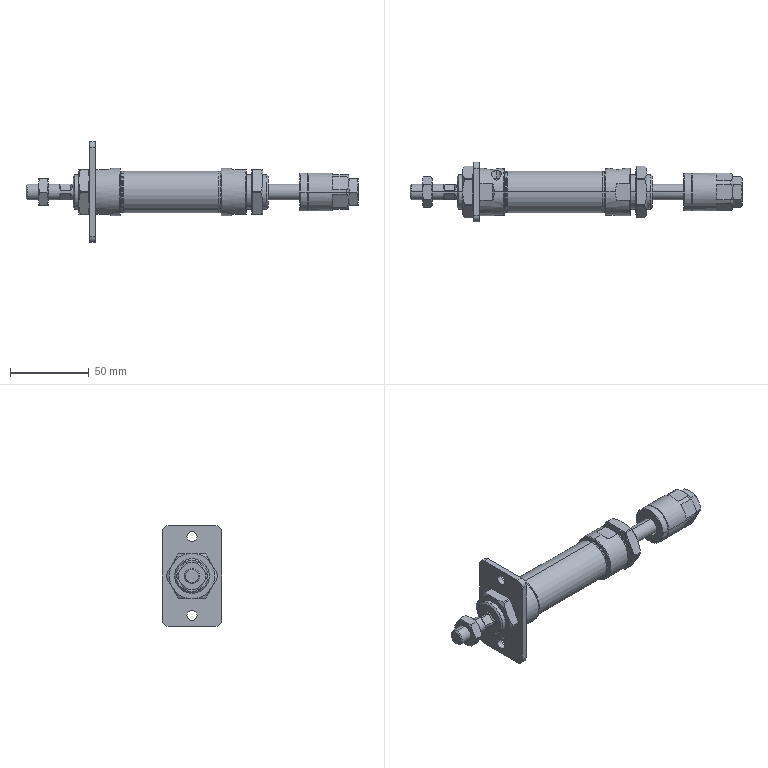Part | STEP file | 8 solids | 272 faces | box 211 x 38 x 64 mm | volume 90003 mm3 | plane 102 | cone 82 | cylinder 74 | torus 14 | commonest cylinder face diameters 33 x12 6.5 x10 10 x8 8 x4 8.566 x4 8.647 x4